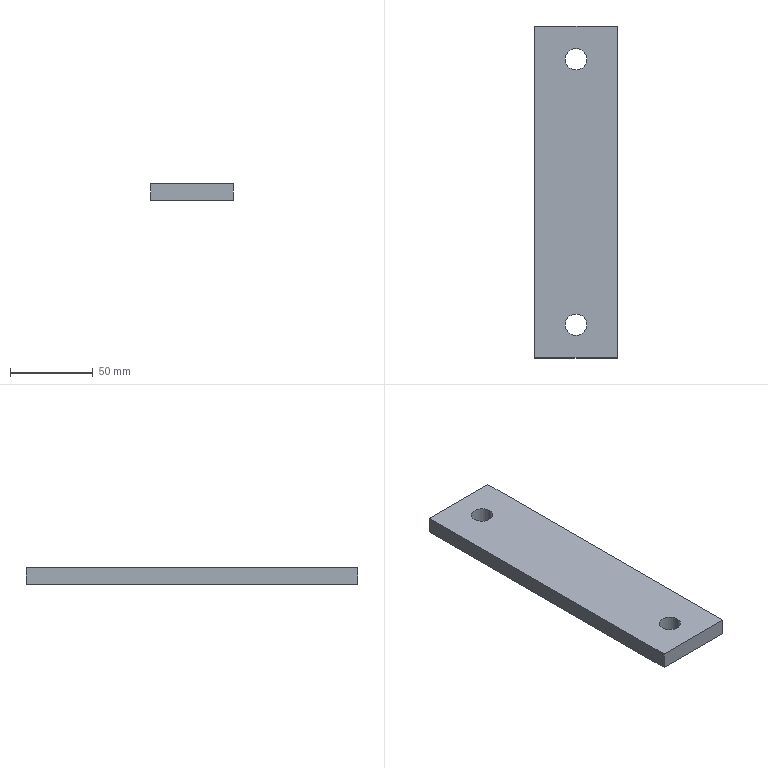Part | SolidWorks | features Extrusion 1 | 1 solid | 10 faces | box 50 x 200 x 10 mm | volume 97345 mm3 | plane 6 | cylinder 4 | commonest cylinder face diameters 13 x4
STEP:
#1=CARTESIAN_POINT('',(-6.5,-80.,10.));
#2=VERTEX_POINT('',#1);
#3=CARTESIAN_POINT('',(6.5,-80.,10.));
#4=VERTEX_POINT('',#3);
#5=CARTESIAN_POINT('',(0.,-80.,10.));
#6=DIRECTION('',(0.,0.,1.));
#7=DIRECTION('',(1.,0.,0.));
#8=AXIS2_PLACEMENT_3D('',#5,#6,#7);
#9=CIRCLE('',#8,6.5);
#10=EDGE_CURVE('',#2,#4,#9,.T.);
#11=ORIENTED_EDGE('',*,*,#10,.T.);
#12=CARTESIAN_POINT('',(6.5,-80.,0.));
#13=VERTEX_POINT('',#12);
#14=CARTESIAN_POINT('',(6.5,-80.,10.));
#15=DIRECTION('',(0.,0.,-1.));
#16=VECTOR('',#15,1000.);
#17=LINE('',#14,#16);
#18=EDGE_CURVE('',#4,#13,#17,.T.);
#19=ORIENTED_EDGE('',*,*,#18,.T.);
#20=CARTESIAN_POINT('',(-6.5,-80.,0.));
#21=VERTEX_POINT('',#20);
#22=CARTESIAN_POINT('',(0.,-80.,0.));
#23=DIRECTION('',(0.,0.,1.));
#24=DIRECTION('',(1.,0.,0.));
#25=AXIS2_PLACEMENT_3D('',#22,#23,#24);
#26=CIRCLE('',#25,6.5);
#27=EDGE_CURVE('',#21,#13,#26,.T.);
#28=ORIENTED_EDGE('',*,*,#27,.F.);
#29=CARTESIAN_POINT('',(-6.5,-80.,10.));
#30=DIRECTION('',(0.,0.,-1.));
#31=VECTOR('',#30,1000.);
#32=LINE('',#29,#31);
#33=EDGE_CURVE('',#2,#21,#32,.T.);
#34=ORIENTED_EDGE('',*,*,#33,.F.);
#35=EDGE_LOOP('',(#11,#19,#28,#34));
#36=FACE_OUTER_BOUND('',#35,.T.);
#37=CARTESIAN_POINT('',(0.,-80.,10.));
#38=DIRECTION('',(0.,0.,-1.));
#39=DIRECTION('',(-1.,0.,0.));
#40=AXIS2_PLACEMENT_3D('',#37,#38,#39);
#41=CYLINDRICAL_SURFACE('',#40,6.5);
#42=ADVANCED_FACE('',(#36),#41,.F.);
#43=CARTESIAN_POINT('',(-6.5,80.,10.));
#44=VERTEX_POINT('',#43);
#45=CARTESIAN_POINT('',(6.5,80.,10.));
#46=VERTEX_POINT('',#45);
#47=CARTESIAN_POINT('',(0.,80.,10.));
#48=DIRECTION('',(0.,0.,1.));
#49=DIRECTION('',(1.,0.,0.));
#50=AXIS2_PLACEMENT_3D('',#47,#48,#49);
#51=CIRCLE('',#50,6.5);
#52=EDGE_CURVE('',#44,#46,#51,.T.);
#53=ORIENTED_EDGE('',*,*,#52,.T.);
#54=CARTESIAN_POINT('',(6.5,80.,0.));
#55=VERTEX_POINT('',#54);
#56=CARTESIAN_POINT('',(6.5,80.,10.));
#57=DIRECTION('',(0.,0.,-1.));
#58=VECTOR('',#57,1000.);
#59=LINE('',#56,#58);
#60=EDGE_CURVE('',#46,#55,#59,.T.);
#61=ORIENTED_EDGE('',*,*,#60,.T.);
#62=CARTESIAN_POINT('',(-6.5,80.,0.));
#63=VERTEX_POINT('',#62);
#64=CARTESIAN_POINT('',(0.,80.,0.));
#65=DIRECTION('',(0.,0.,1.));
#66=DIRECTION('',(1.,0.,0.));
#67=AXIS2_PLACEMENT_3D('',#64,#65,#66);
#68=CIRCLE('',#67,6.5);
#69=EDGE_CURVE('',#63,#55,#68,.T.);
#70=ORIENTED_EDGE('',*,*,#69,.F.);
#71=CARTESIAN_POINT('',(-6.5,80.,10.));
#72=DIRECTION('',(0.,0.,-1.));
#73=VECTOR('',#72,1000.);
#74=LINE('',#71,#73);
#75=EDGE_CURVE('',#44,#63,#74,.T.);
#76=ORIENTED_EDGE('',*,*,#75,.F.);
#77=EDGE_LOOP('',(#53,#61,#70,#76));
#78=FACE_OUTER_BOUND('',#77,.T.);
#79=CARTESIAN_POINT('',(0.,80.,10.));
#80=DIRECTION('',(0.,0.,-1.));
#81=DIRECTION('',(-1.,0.,0.));
#82=AXIS2_PLACEMENT_3D('',#79,#80,#81);
#83=CYLINDRICAL_SURFACE('',#82,6.5);
#84=ADVANCED_FACE('',(#78),#83,.F.);
#85=ORIENTED_EDGE('',*,*,#52,.F.);
#86=CARTESIAN_POINT('',(0.,80.,10.));
#87=DIRECTION('',(0.,0.,1.));
#88=DIRECTION('',(1.,0.,0.));
#89=AXIS2_PLACEMENT_3D('',#86,#87,#88);
#90=CIRCLE('',#89,6.5);
#91=EDGE_CURVE('',#46,#44,#90,.T.);
#92=ORIENTED_EDGE('',*,*,#91,.F.);
#93=EDGE_LOOP('',(#85,#92));
#94=FACE_BOUND('',#93,.T.);
#95=CARTESIAN_POINT('',(25.,-100.,10.));
#96=VERTEX_POINT('',#95);
#97=CARTESIAN_POINT('',(25.,100.,10.));
#98=VERTEX_POINT('',#97);
#99=CARTESIAN_POINT('',(25.,100.,10.));
#100=DIRECTION('',(0.,1.,0.));
#101=VECTOR('',#100,1000.);
#102=LINE('',#99,#101);
#103=EDGE_CURVE('',#96,#98,#102,.T.);
#104=ORIENTED_EDGE('',*,*,#103,.T.);
#105=CARTESIAN_POINT('',(-25.,100.,10.));
#106=VERTEX_POINT('',#105);
#107=CARTESIAN_POINT('',(-25.,100.,10.));
#108=DIRECTION('',(-1.,0.,0.));
#109=VECTOR('',#108,1000.);
#110=LINE('',#107,#109);
#111=EDGE_CURVE('',#98,#106,#110,.T.);
#112=ORIENTED_EDGE('',*,*,#111,.T.);
#113=CARTESIAN_POINT('',(-25.,-100.,10.));
#114=VERTEX_POINT('',#113);
#115=CARTESIAN_POINT('',(-25.,100.,10.));
#116=DIRECTION('',(0.,-1.,0.));
#117=VECTOR('',#116,1000.);
#118=LINE('',#115,#117);
#119=EDGE_CURVE('',#106,#114,#118,.T.);
#120=ORIENTED_EDGE('',*,*,#119,.T.);
#121=CARTESIAN_POINT('',(-25.,-100.,10.));
#122=DIRECTION('',(1.,0.,0.));
#123=VECTOR('',#122,1000.);
#124=LINE('',#121,#123);
#125=EDGE_CURVE('',#114,#96,#124,.T.);
#126=ORIENTED_EDGE('',*,*,#125,.T.);
#127=EDGE_LOOP('',(#104,#112,#120,#126));
#128=FACE_OUTER_BOUND('',#127,.T.);
#129=ORIENTED_EDGE('',*,*,#10,.F.);
#130=CARTESIAN_POINT('',(0.,-80.,10.));
#131=DIRECTION('',(0.,0.,1.));
#132=DIRECTION('',(1.,0.,0.));
#133=AXIS2_PLACEMENT_3D('',#130,#131,#132);
#134=CIRCLE('',#133,6.5);
#135=EDGE_CURVE('',#4,#2,#134,.T.);
#136=ORIENTED_EDGE('',*,*,#135,.F.);
#137=EDGE_LOOP('',(#129,#136));
#138=FACE_BOUND('',#137,.T.);
#139=CARTESIAN_POINT('',(0.,0.,10.));
#140=DIRECTION('',(0.,0.,1.));
#141=DIRECTION('',(1.,0.,0.));
#142=AXIS2_PLACEMENT_3D('',#139,#140,#141);
#143=PLANE('',#142);
#144=ADVANCED_FACE('',(#94,#128,#138),#143,.T.);
#145=CARTESIAN_POINT('',(25.,-100.,0.));
#146=VERTEX_POINT('',#145);
#147=CARTESIAN_POINT('',(25.,100.,0.));
#148=VERTEX_POINT('',#147);
#149=CARTESIAN_POINT('',(25.,100.,0.));
#150=DIRECTION('',(0.,1.,0.));
#151=VECTOR('',#150,1000.);
#152=LINE('',#149,#151);
#153=EDGE_CURVE('',#146,#148,#152,.T.);
#154=ORIENTED_EDGE('',*,*,#153,.F.);
#155=CARTESIAN_POINT('',(-25.,-100.,0.));
#156=VERTEX_POINT('',#155);
#157=CARTESIAN_POINT('',(-25.,-100.,0.));
#158=DIRECTION('',(1.,0.,0.));
#159=VECTOR('',#158,1000.);
#160=LINE('',#157,#159);
#161=EDGE_CURVE('',#156,#146,#160,.T.);
#162=ORIENTED_EDGE('',*,*,#161,.F.);
#163=CARTESIAN_POINT('',(-25.,100.,0.));
#164=VERTEX_POINT('',#163);
#165=CARTESIAN_POINT('',(-25.,100.,0.));
#166=DIRECTION('',(0.,-1.,0.));
#167=VECTOR('',#166,1000.);
#168=LINE('',#165,#167);
#169=EDGE_CURVE('',#164,#156,#168,.T.);
#170=ORIENTED_EDGE('',*,*,#169,.F.);
#171=CARTESIAN_POINT('',(-25.,100.,0.));
#172=DIRECTION('',(-1.,0.,0.));
#173=VECTOR('',#172,1000.);
#174=LINE('',#171,#173);
#175=EDGE_CURVE('',#148,#164,#174,.T.);
#176=ORIENTED_EDGE('',*,*,#175,.F.);
#177=EDGE_LOOP('',(#154,#162,#170,#176));
#178=FACE_OUTER_BOUND('',#177,.T.);
#179=ORIENTED_EDGE('',*,*,#69,.T.);
#180=CARTESIAN_POINT('',(0.,80.,0.));
#181=DIRECTION('',(0.,0.,1.));
#182=DIRECTION('',(1.,0.,0.));
#183=AXIS2_PLACEMENT_3D('',#180,#181,#182);
#184=CIRCLE('',#183,6.5);
#185=EDGE_CURVE('',#55,#63,#184,.T.);
#186=ORIENTED_EDGE('',*,*,#185,.T.);
#187=EDGE_LOOP('',(#179,#186));
#188=FACE_BOUND('',#187,.T.);
#189=ORIENTED_EDGE('',*,*,#27,.T.);
#190=CARTESIAN_POINT('',(0.,-80.,0.));
#191=DIRECTION('',(0.,0.,1.));
#192=DIRECTION('',(1.,0.,0.));
#193=AXIS2_PLACEMENT_3D('',#190,#191,#192);
#194=CIRCLE('',#193,6.5);
#195=EDGE_CURVE('',#13,#21,#194,.T.);
#196=ORIENTED_EDGE('',*,*,#195,.T.);
#197=EDGE_LOOP('',(#189,#196));
#198=FACE_BOUND('',#197,.T.);
#199=CARTESIAN_POINT('',(0.,0.,0.));
#200=DIRECTION('',(0.,0.,1.));
#201=DIRECTION('',(1.,0.,0.));
#202=AXIS2_PLACEMENT_3D('',#199,#200,#201);
#203=PLANE('',#202);
#204=ADVANCED_FACE('',(#178,#188,#198),#203,.F.);
#205=ORIENTED_EDGE('',*,*,#153,.T.);
#206=CARTESIAN_POINT('',(25.,100.,10.));
#207=DIRECTION('',(0.,0.,-1.));
#208=VECTOR('',#207,1000.);
#209=LINE('',#206,#208);
#210=EDGE_CURVE('',#98,#148,#209,.T.);
#211=ORIENTED_EDGE('',*,*,#210,.F.);
#212=ORIENTED_EDGE('',*,*,#103,.F.);
#213=CARTESIAN_POINT('',(25.,-100.,10.));
#214=DIRECTION('',(0.,0.,-1.));
#215=VECTOR('',#214,1000.);
#216=LINE('',#213,#215);
#217=EDGE_CURVE('',#96,#146,#216,.T.);
#218=ORIENTED_EDGE('',*,*,#217,.T.);
#219=EDGE_LOOP('',(#205,#211,#212,#218));
#220=FACE_OUTER_BOUND('',#219,.T.);
#221=CARTESIAN_POINT('',(25.,100.,10.));
#222=DIRECTION('',(-1.,0.,0.));
#223=DIRECTION('',(0.,-1.,0.));
#224=AXIS2_PLACEMENT_3D('',#221,#222,#223);
#225=PLANE('',#224);
#226=ADVANCED_FACE('',(#220),#225,.F.);
#227=ORIENTED_EDGE('',*,*,#175,.T.);
#228=CARTESIAN_POINT('',(-25.,100.,10.));
#229=DIRECTION('',(0.,0.,-1.));
#230=VECTOR('',#229,1000.);
#231=LINE('',#228,#230);
#232=EDGE_CURVE('',#106,#164,#231,.T.);
#233=ORIENTED_EDGE('',*,*,#232,.F.);
#234=ORIENTED_EDGE('',*,*,#111,.F.);
#235=ORIENTED_EDGE('',*,*,#210,.T.);
#236=EDGE_LOOP('',(#227,#233,#234,#235));
#237=FACE_OUTER_BOUND('',#236,.T.);
#238=CARTESIAN_POINT('',(-25.,100.,10.));
#239=DIRECTION('',(0.,-1.,0.));
#240=DIRECTION('',(0.,0.,-1.));
#241=AXIS2_PLACEMENT_3D('',#238,#239,#240);
#242=PLANE('',#241);
#243=ADVANCED_FACE('',(#237),#242,.F.);
#244=ORIENTED_EDGE('',*,*,#169,.T.);
#245=CARTESIAN_POINT('',(-25.,-100.,10.));
#246=DIRECTION('',(0.,0.,-1.));
#247=VECTOR('',#246,1000.);
#248=LINE('',#245,#247);
#249=EDGE_CURVE('',#114,#156,#248,.T.);
#250=ORIENTED_EDGE('',*,*,#249,.F.);
#251=ORIENTED_EDGE('',*,*,#119,.F.);
#252=ORIENTED_EDGE('',*,*,#232,.T.);
#253=EDGE_LOOP('',(#244,#250,#251,#252));
#254=FACE_OUTER_BOUND('',#253,.T.);
#255=CARTESIAN_POINT('',(-25.,100.,10.));
#256=DIRECTION('',(1.,0.,0.));
#257=DIRECTION('',(0.,1.,0.));
#258=AXIS2_PLACEMENT_3D('',#255,#256,#257);
#259=PLANE('',#258);
#260=ADVANCED_FACE('',(#254),#259,.F.);
#261=ORIENTED_EDGE('',*,*,#161,.T.);
#262=ORIENTED_EDGE('',*,*,#217,.F.);
#263=ORIENTED_EDGE('',*,*,#125,.F.);
#264=ORIENTED_EDGE('',*,*,#249,.T.);
#265=EDGE_LOOP('',(#261,#262,#263,#264));
#266=FACE_OUTER_BOUND('',#265,.T.);
#267=CARTESIAN_POINT('',(-25.,-100.,10.));
#268=DIRECTION('',(0.,1.,0.));
#269=DIRECTION('',(0.,0.,1.));
#270=AXIS2_PLACEMENT_3D('',#267,#268,#269);
#271=PLANE('',#270);
#272=ADVANCED_FACE('',(#266),#271,.F.);
#273=ORIENTED_EDGE('',*,*,#60,.F.);
#274=ORIENTED_EDGE('',*,*,#91,.T.);
#275=ORIENTED_EDGE('',*,*,#75,.T.);
#276=ORIENTED_EDGE('',*,*,#185,.F.);
#277=EDGE_LOOP('',(#273,#274,#275,#276));
#278=FACE_OUTER_BOUND('',#277,.T.);
#279=CARTESIAN_POINT('',(0.,80.,10.));
#280=DIRECTION('',(0.,0.,-1.));
#281=DIRECTION('',(-1.,0.,0.));
#282=AXIS2_PLACEMENT_3D('',#279,#280,#281);
#283=CYLINDRICAL_SURFACE('',#282,6.5);
#284=ADVANCED_FACE('',(#278),#283,.F.);
#285=ORIENTED_EDGE('',*,*,#18,.F.);
#286=ORIENTED_EDGE('',*,*,#135,.T.);
#287=ORIENTED_EDGE('',*,*,#33,.T.);
#288=ORIENTED_EDGE('',*,*,#195,.F.);
#289=EDGE_LOOP('',(#285,#286,#287,#288));
#290=FACE_OUTER_BOUND('',#289,.T.);
#291=CARTESIAN_POINT('',(0.,-80.,10.));
#292=DIRECTION('',(0.,0.,-1.));
#293=DIRECTION('',(-1.,0.,0.));
#294=AXIS2_PLACEMENT_3D('',#291,#292,#293);
#295=CYLINDRICAL_SURFACE('',#294,6.5);
#296=ADVANCED_FACE('',(#290),#295,.F.);
#297=CLOSED_SHELL('',(#42,#84,#144,#204,#226,#243,#260,#272,#284,#296));
#298=MANIFOLD_SOLID_BREP('',#297);
#299=CARTESIAN_POINT('',(0.,0.,0.));
#300=DIRECTION('',(0.,0.,1.));
#301=DIRECTION('',(1.,0.,0.));
#302=AXIS2_PLACEMENT_3D('',#299,#300,#301);
#303=(LENGTH_UNIT()NAMED_UNIT(*)SI_UNIT(.MILLI.,.METRE.));
#304=UNCERTAINTY_MEASURE_WITH_UNIT(LENGTH_MEASURE(0.00001),#303,'','');
#305=(NAMED_UNIT(*)PLANE_ANGLE_UNIT()SI_UNIT($,.RADIAN.));
#306=(NAMED_UNIT(*)SI_UNIT($,.STERADIAN.)SOLID_ANGLE_UNIT());
#307=(GEOMETRIC_REPRESENTATION_CONTEXT(3)GLOBAL_UNCERTAINTY_ASSIGNED_CONTEXT((#304))GLOBAL_UNIT_ASSIGNED_CONTEXT((#303,#305,#306))REPRESENTATION_CONTEXT('',''));
#308=ADVANCED_BREP_SHAPE_REPRESENTATION('',(#298,#302),#307);